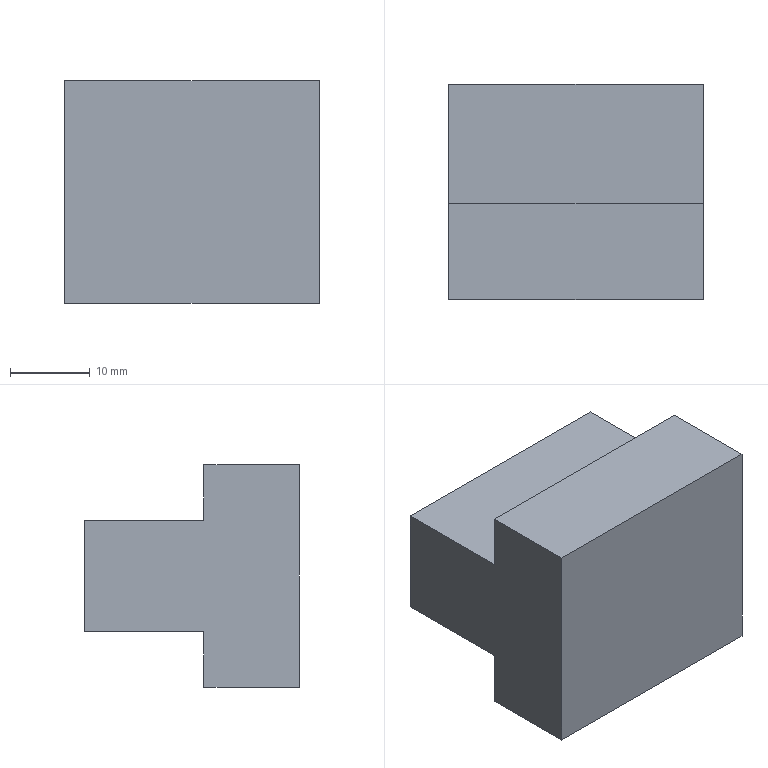Part | STEP file | PN_0009 gripper MHS3-80D | 1 solid | 18 faces | box 32 x 27 x 28 mm | volume 16863 mm3 | plane 10 | cylinder 4 | cone 4 | commonest cylinder face diameters 5 x4
STEP:
#1=CARTESIAN_POINT('',(0.,0.,0.));
#2=DIRECTION('',(0.,0.,1.));
#3=DIRECTION('',(1.,0.,0.));
#4=AXIS2_PLACEMENT_3D('',#1,#2,#3);
#5=CARTESIAN_POINT('',(-10.,12.,2.5));
#6=VERTEX_POINT('',#5);
#7=CARTESIAN_POINT('',(-10.,27.,2.5));
#8=VERTEX_POINT('',#7);
#9=CARTESIAN_POINT('',(-10.,27.,2.5));
#10=DIRECTION('',(0.,1.,0.));
#11=VECTOR('',#10,1.);
#12=LINE('',#9,#11);
#13=CARTESIAN_POINT('',(-10.,27.,0.));
#14=DIRECTION('',(0.,1.,0.));
#15=DIRECTION('',(0.,0.,1.));
#16=AXIS2_PLACEMENT_3D('',#13,#14,#15);
#17=CYLINDRICAL_SURFACE('',#16,2.5);
#18=CARTESIAN_POINT('',(6.283,0.));
#19=DIRECTION('',(0.,1.));
#20=VECTOR('',#19,1.);
#21=LINE('',#18,#20);
#22=(GEOMETRIC_REPRESENTATION_CONTEXT(2)PARAMETRIC_REPRESENTATION_CONTEXT()REPRESENTATION_CONTEXT('',''));
#23=DEFINITIONAL_REPRESENTATION('',(#21),#22);
#24=PCURVE('',#17,#23);
#25=CARTESIAN_POINT('',(-10.,27.,0.));
#26=DIRECTION('',(0.,1.,0.));
#27=DIRECTION('',(0.,0.,1.));
#28=AXIS2_PLACEMENT_3D('',#25,#26,#27);
#29=CYLINDRICAL_SURFACE('',#28,2.5);
#30=CARTESIAN_POINT('',(0.,0.));
#31=DIRECTION('',(0.,1.));
#32=VECTOR('',#31,1.);
#33=LINE('',#30,#32);
#34=(GEOMETRIC_REPRESENTATION_CONTEXT(2)PARAMETRIC_REPRESENTATION_CONTEXT()REPRESENTATION_CONTEXT('',''));
#35=DEFINITIONAL_REPRESENTATION('',(#33),#34);
#36=PCURVE('',#29,#35);
#37=SURFACE_CURVE('',#12,(#24,#36),.PCURVE_S1.);
#38=EDGE_CURVE('',#6,#8,#37,.T.);
#39=ORIENTED_EDGE('',*,*,#38,.T.);
#40=CARTESIAN_POINT('',(-10.,27.,-2.5));
#41=VERTEX_POINT('',#40);
#42=CARTESIAN_POINT('',(-10.,27.,0.));
#43=DIRECTION('',(0.,1.,0.));
#44=DIRECTION('',(0.,0.,1.));
#45=AXIS2_PLACEMENT_3D('',#42,#43,#44);
#46=CIRCLE('',#45,2.5);
#47=CARTESIAN_POINT('',(0.,0.));
#48=DIRECTION('',(1.,0.));
#49=VECTOR('',#48,1.);
#50=LINE('',#47,#49);
#51=(GEOMETRIC_REPRESENTATION_CONTEXT(2)PARAMETRIC_REPRESENTATION_CONTEXT()REPRESENTATION_CONTEXT('',''));
#52=DEFINITIONAL_REPRESENTATION('',(#50),#51);
#53=PCURVE('',#17,#52);
#54=CARTESIAN_POINT('',(16.,27.,7.));
#55=DIRECTION('',(0.,-1.,0.));
#56=DIRECTION('',(0.,0.,-1.));
#57=AXIS2_PLACEMENT_3D('',#54,#55,#56);
#58=PLANE('',#57);
#59=CARTESIAN_POINT('',(4.5,-26.));
#60=CARTESIAN_POINT('',(4.5,-21.67));
#61=CARTESIAN_POINT('',(8.25,-23.835));
#62=CARTESIAN_POINT('',(12.,-26.));
#63=CARTESIAN_POINT('',(8.25,-28.165));
#64=CARTESIAN_POINT('',(4.5,-30.33));
#65=CARTESIAN_POINT('',(4.5,-26.));
#66=(BOUNDED_CURVE()B_SPLINE_CURVE(2,(#59,#60,#61,#62,#63,#64,#65),.UNSPECIFIED.,.T.,.F.)B_SPLINE_CURVE_WITH_KNOTS((1,2,2,2,2,1),(-2.094,0.,2.094,4.189,6.283,8.378),.UNSPECIFIED.)CURVE()GEOMETRIC_REPRESENTATION_ITEM()RATIONAL_B_SPLINE_CURVE((1.,0.5,1.,0.5,1.,0.5,1.))REPRESENTATION_ITEM(''));
#67=(GEOMETRIC_REPRESENTATION_CONTEXT(2)PARAMETRIC_REPRESENTATION_CONTEXT()REPRESENTATION_CONTEXT('',''));
#68=DEFINITIONAL_REPRESENTATION('',(#66),#67);
#69=PCURVE('',#58,#68);
#70=SURFACE_CURVE('',#46,(#53,#69),.PCURVE_S1.);
#71=EDGE_CURVE('',#41,#8,#70,.T.);
#72=ORIENTED_EDGE('',*,*,#71,.F.);
#73=CARTESIAN_POINT('',(-10.,12.,-2.5));
#74=VERTEX_POINT('',#73);
#75=CARTESIAN_POINT('',(-10.,27.,-2.5));
#76=DIRECTION('',(0.,1.,0.));
#77=VECTOR('',#76,1.);
#78=LINE('',#75,#77);
#79=CARTESIAN_POINT('',(3.142,0.));
#80=DIRECTION('',(0.,1.));
#81=VECTOR('',#80,1.);
#82=LINE('',#79,#81);
#83=(GEOMETRIC_REPRESENTATION_CONTEXT(2)PARAMETRIC_REPRESENTATION_CONTEXT()REPRESENTATION_CONTEXT('',''));
#84=DEFINITIONAL_REPRESENTATION('',(#82),#83);
#85=PCURVE('',#17,#84);
#86=CARTESIAN_POINT('',(3.142,0.));
#87=DIRECTION('',(0.,1.));
#88=VECTOR('',#87,1.);
#89=LINE('',#86,#88);
#90=(GEOMETRIC_REPRESENTATION_CONTEXT(2)PARAMETRIC_REPRESENTATION_CONTEXT()REPRESENTATION_CONTEXT('',''));
#91=DEFINITIONAL_REPRESENTATION('',(#89),#90);
#92=PCURVE('',#29,#91);
#93=SURFACE_CURVE('',#78,(#85,#92),.PCURVE_S1.);
#94=EDGE_CURVE('',#74,#41,#93,.T.);
#95=ORIENTED_EDGE('',*,*,#94,.F.);
#96=CARTESIAN_POINT('',(-10.,12.,0.));
#97=DIRECTION('',(0.,1.,0.));
#98=DIRECTION('',(0.,0.,1.));
#99=AXIS2_PLACEMENT_3D('',#96,#97,#98);
#100=CIRCLE('',#99,2.5);
#101=CARTESIAN_POINT('',(0.,-15.));
#102=DIRECTION('',(1.,0.));
#103=VECTOR('',#102,1.);
#104=LINE('',#101,#103);
#105=(GEOMETRIC_REPRESENTATION_CONTEXT(2)PARAMETRIC_REPRESENTATION_CONTEXT()REPRESENTATION_CONTEXT('',''));
#106=DEFINITIONAL_REPRESENTATION('',(#104),#105);
#107=PCURVE('',#17,#106);
#108=CARTESIAN_POINT('',(-10.,12.,0.));
#109=DIRECTION('',(0.,1.,0.));
#110=DIRECTION('',(0.,0.,1.));
#111=AXIS2_PLACEMENT_3D('',#108,#109,#110);
#112=CONICAL_SURFACE('',#111,2.5,1.03);
#113=CARTESIAN_POINT('',(0.,0.));
#114=DIRECTION('',(1.,0.));
#115=VECTOR('',#114,1.);
#116=LINE('',#113,#115);
#117=(GEOMETRIC_REPRESENTATION_CONTEXT(2)PARAMETRIC_REPRESENTATION_CONTEXT()REPRESENTATION_CONTEXT('',''));
#118=DEFINITIONAL_REPRESENTATION('',(#116),#117);
#119=PCURVE('',#112,#118);
#120=SURFACE_CURVE('',#100,(#107,#119),.PCURVE_S1.);
#121=EDGE_CURVE('',#74,#6,#120,.T.);
#122=ORIENTED_EDGE('',*,*,#121,.T.);
#123=EDGE_LOOP('',(#39,#72,#95,#122));
#124=FACE_BOUND('',#123,.F.);
#125=ADVANCED_FACE('',(#124),#17,.F.);
#126=ORIENTED_EDGE('',*,*,#121,.F.);
#127=CARTESIAN_POINT('',(-10.,10.498,0.));
#128=VERTEX_POINT('',#127);
#129=CARTESIAN_POINT('',(-10.,12.,-2.5));
#130=DIRECTION('',(0.,0.515,-0.8572));
#131=VECTOR('',#130,1.);
#132=LINE('',#129,#131);
#133=CARTESIAN_POINT('',(3.142,0.));
#134=DIRECTION('',(0.,1.));
#135=VECTOR('',#134,1.);
#136=LINE('',#133,#135);
#137=(GEOMETRIC_REPRESENTATION_CONTEXT(2)PARAMETRIC_REPRESENTATION_CONTEXT()REPRESENTATION_CONTEXT('',''));
#138=DEFINITIONAL_REPRESENTATION('',(#136),#137);
#139=PCURVE('',#112,#138);
#140=CARTESIAN_POINT('',(-10.,12.,0.));
#141=DIRECTION('',(0.,1.,0.));
#142=DIRECTION('',(0.,0.,1.));
#143=AXIS2_PLACEMENT_3D('',#140,#141,#142);
#144=CONICAL_SURFACE('',#143,2.5,1.03);
#145=CARTESIAN_POINT('',(3.142,0.));
#146=DIRECTION('',(0.,1.));
#147=VECTOR('',#146,1.);
#148=LINE('',#145,#147);
#149=(GEOMETRIC_REPRESENTATION_CONTEXT(2)PARAMETRIC_REPRESENTATION_CONTEXT()REPRESENTATION_CONTEXT('',''));
#150=DEFINITIONAL_REPRESENTATION('',(#148),#149);
#151=PCURVE('',#144,#150);
#152=SURFACE_CURVE('',#132,(#139,#151),.PCURVE_S1.);
#153=EDGE_CURVE('',#128,#74,#152,.T.);
#154=ORIENTED_EDGE('',*,*,#153,.F.);
#155=CARTESIAN_POINT('',(-10.,12.,2.5));
#156=DIRECTION('',(0.,0.515,0.8572));
#157=VECTOR('',#156,1.);
#158=LINE('',#155,#157);
#159=CARTESIAN_POINT('',(6.283,0.));
#160=DIRECTION('',(0.,1.));
#161=VECTOR('',#160,1.);
#162=LINE('',#159,#161);
#163=(GEOMETRIC_REPRESENTATION_CONTEXT(2)PARAMETRIC_REPRESENTATION_CONTEXT()REPRESENTATION_CONTEXT('',''));
#164=DEFINITIONAL_REPRESENTATION('',(#162),#163);
#165=PCURVE('',#112,#164);
#166=CARTESIAN_POINT('',(0.,0.));
#167=DIRECTION('',(0.,1.));
#168=VECTOR('',#167,1.);
#169=LINE('',#166,#168);
#170=(GEOMETRIC_REPRESENTATION_CONTEXT(2)PARAMETRIC_REPRESENTATION_CONTEXT()REPRESENTATION_CONTEXT('',''));
#171=DEFINITIONAL_REPRESENTATION('',(#169),#170);
#172=PCURVE('',#144,#171);
#173=SURFACE_CURVE('',#158,(#165,#172),.PCURVE_S1.);
#174=EDGE_CURVE('',#128,#6,#173,.T.);
#175=ORIENTED_EDGE('',*,*,#174,.T.);
#176=EDGE_LOOP('',(#126,#154,#175));
#177=FACE_BOUND('',#176,.F.);
#178=ADVANCED_FACE('',(#177),#112,.F.);
#179=CARTESIAN_POINT('',(10.,12.,2.5));
#180=VERTEX_POINT('',#179);
#181=CARTESIAN_POINT('',(10.,27.,2.5));
#182=VERTEX_POINT('',#181);
#183=CARTESIAN_POINT('',(10.,27.,2.5));
#184=DIRECTION('',(0.,1.,0.));
#185=VECTOR('',#184,1.);
#186=LINE('',#183,#185);
#187=CARTESIAN_POINT('',(10.,27.,0.));
#188=DIRECTION('',(0.,1.,0.));
#189=DIRECTION('',(0.,0.,1.));
#190=AXIS2_PLACEMENT_3D('',#187,#188,#189);
#191=CYLINDRICAL_SURFACE('',#190,2.5);
#192=CARTESIAN_POINT('',(6.283,0.));
#193=DIRECTION('',(0.,1.));
#194=VECTOR('',#193,1.);
#195=LINE('',#192,#194);
#196=(GEOMETRIC_REPRESENTATION_CONTEXT(2)PARAMETRIC_REPRESENTATION_CONTEXT()REPRESENTATION_CONTEXT('',''));
#197=DEFINITIONAL_REPRESENTATION('',(#195),#196);
#198=PCURVE('',#191,#197);
#199=CARTESIAN_POINT('',(10.,27.,0.));
#200=DIRECTION('',(0.,1.,0.));
#201=DIRECTION('',(0.,0.,1.));
#202=AXIS2_PLACEMENT_3D('',#199,#200,#201);
#203=CYLINDRICAL_SURFACE('',#202,2.5);
#204=CARTESIAN_POINT('',(0.,0.));
#205=DIRECTION('',(0.,1.));
#206=VECTOR('',#205,1.);
#207=LINE('',#204,#206);
#208=(GEOMETRIC_REPRESENTATION_CONTEXT(2)PARAMETRIC_REPRESENTATION_CONTEXT()REPRESENTATION_CONTEXT('',''));
#209=DEFINITIONAL_REPRESENTATION('',(#207),#208);
#210=PCURVE('',#203,#209);
#211=SURFACE_CURVE('',#186,(#198,#210),.PCURVE_S1.);
#212=EDGE_CURVE('',#180,#182,#211,.T.);
#213=ORIENTED_EDGE('',*,*,#212,.T.);
#214=CARTESIAN_POINT('',(10.,27.,-2.5));
#215=VERTEX_POINT('',#214);
#216=CARTESIAN_POINT('',(10.,27.,0.));
#217=DIRECTION('',(0.,1.,0.));
#218=DIRECTION('',(0.,0.,1.));
#219=AXIS2_PLACEMENT_3D('',#216,#217,#218);
#220=CIRCLE('',#219,2.5);
#221=CARTESIAN_POINT('',(0.,0.));
#222=DIRECTION('',(1.,0.));
#223=VECTOR('',#222,1.);
#224=LINE('',#221,#223);
#225=(GEOMETRIC_REPRESENTATION_CONTEXT(2)PARAMETRIC_REPRESENTATION_CONTEXT()REPRESENTATION_CONTEXT('',''));
#226=DEFINITIONAL_REPRESENTATION('',(#224),#225);
#227=PCURVE('',#191,#226);
#228=CARTESIAN_POINT('',(4.5,-6.));
#229=CARTESIAN_POINT('',(4.5,-1.67));
#230=CARTESIAN_POINT('',(8.25,-3.835));
#231=CARTESIAN_POINT('',(12.,-6.));
#232=CARTESIAN_POINT('',(8.25,-8.165));
#233=CARTESIAN_POINT('',(4.5,-10.33));
#234=CARTESIAN_POINT('',(4.5,-6.));
#235=(BOUNDED_CURVE()B_SPLINE_CURVE(2,(#228,#229,#230,#231,#232,#233,#234),.UNSPECIFIED.,.T.,.F.)B_SPLINE_CURVE_WITH_KNOTS((1,2,2,2,2,1),(-2.094,0.,2.094,4.189,6.283,8.378),.UNSPECIFIED.)CURVE()GEOMETRIC_REPRESENTATION_ITEM()RATIONAL_B_SPLINE_CURVE((1.,0.5,1.,0.5,1.,0.5,1.))REPRESENTATION_ITEM(''));
#236=(GEOMETRIC_REPRESENTATION_CONTEXT(2)PARAMETRIC_REPRESENTATION_CONTEXT()REPRESENTATION_CONTEXT('',''));
#237=DEFINITIONAL_REPRESENTATION('',(#235),#236);
#238=PCURVE('',#58,#237);
#239=SURFACE_CURVE('',#220,(#227,#238),.PCURVE_S1.);
#240=EDGE_CURVE('',#215,#182,#239,.T.);
#241=ORIENTED_EDGE('',*,*,#240,.F.);
#242=CARTESIAN_POINT('',(10.,12.,-2.5));
#243=VERTEX_POINT('',#242);
#244=CARTESIAN_POINT('',(10.,27.,-2.5));
#245=DIRECTION('',(0.,1.,0.));
#246=VECTOR('',#245,1.);
#247=LINE('',#244,#246);
#248=CARTESIAN_POINT('',(3.142,0.));
#249=DIRECTION('',(0.,1.));
#250=VECTOR('',#249,1.);
#251=LINE('',#248,#250);
#252=(GEOMETRIC_REPRESENTATION_CONTEXT(2)PARAMETRIC_REPRESENTATION_CONTEXT()REPRESENTATION_CONTEXT('',''));
#253=DEFINITIONAL_REPRESENTATION('',(#251),#252);
#254=PCURVE('',#191,#253);
#255=CARTESIAN_POINT('',(3.142,0.));
#256=DIRECTION('',(0.,1.));
#257=VECTOR('',#256,1.);
#258=LINE('',#255,#257);
#259=(GEOMETRIC_REPRESENTATION_CONTEXT(2)PARAMETRIC_REPRESENTATION_CONTEXT()REPRESENTATION_CONTEXT('',''));
#260=DEFINITIONAL_REPRESENTATION('',(#258),#259);
#261=PCURVE('',#203,#260);
#262=SURFACE_CURVE('',#247,(#254,#261),.PCURVE_S1.);
#263=EDGE_CURVE('',#243,#215,#262,.T.);
#264=ORIENTED_EDGE('',*,*,#263,.F.);
#265=CARTESIAN_POINT('',(10.,12.,0.));
#266=DIRECTION('',(0.,1.,0.));
#267=DIRECTION('',(0.,0.,1.));
#268=AXIS2_PLACEMENT_3D('',#265,#266,#267);
#269=CIRCLE('',#268,2.5);
#270=CARTESIAN_POINT('',(0.,-15.));
#271=DIRECTION('',(1.,0.));
#272=VECTOR('',#271,1.);
#273=LINE('',#270,#272);
#274=(GEOMETRIC_REPRESENTATION_CONTEXT(2)PARAMETRIC_REPRESENTATION_CONTEXT()REPRESENTATION_CONTEXT('',''));
#275=DEFINITIONAL_REPRESENTATION('',(#273),#274);
#276=PCURVE('',#191,#275);
#277=CARTESIAN_POINT('',(10.,12.,0.));
#278=DIRECTION('',(0.,1.,0.));
#279=DIRECTION('',(0.,0.,1.));
#280=AXIS2_PLACEMENT_3D('',#277,#278,#279);
#281=CONICAL_SURFACE('',#280,2.5,1.03);
#282=CARTESIAN_POINT('',(0.,0.));
#283=DIRECTION('',(1.,0.));
#284=VECTOR('',#283,1.);
#285=LINE('',#282,#284);
#286=(GEOMETRIC_REPRESENTATION_CONTEXT(2)PARAMETRIC_REPRESENTATION_CONTEXT()REPRESENTATION_CONTEXT('',''));
#287=DEFINITIONAL_REPRESENTATION('',(#285),#286);
#288=PCURVE('',#281,#287);
#289=SURFACE_CURVE('',#269,(#276,#288),.PCURVE_S1.);
#290=EDGE_CURVE('',#243,#180,#289,.T.);
#291=ORIENTED_EDGE('',*,*,#290,.T.);
#292=EDGE_LOOP('',(#213,#241,#264,#291));
#293=FACE_BOUND('',#292,.F.);
#294=ADVANCED_FACE('',(#293),#191,.F.);
#295=ORIENTED_EDGE('',*,*,#290,.F.);
#296=CARTESIAN_POINT('',(10.,10.498,0.));
#297=VERTEX_POINT('',#296);
#298=CARTESIAN_POINT('',(10.,12.,-2.5));
#299=DIRECTION('',(0.,0.515,-0.8572));
#300=VECTOR('',#299,1.);
#301=LINE('',#298,#300);
#302=CARTESIAN_POINT('',(3.142,0.));
#303=DIRECTION('',(0.,1.));
#304=VECTOR('',#303,1.);
#305=LINE('',#302,#304);
#306=(GEOMETRIC_REPRESENTATION_CONTEXT(2)PARAMETRIC_REPRESENTATION_CONTEXT()REPRESENTATION_CONTEXT('',''));
#307=DEFINITIONAL_REPRESENTATION('',(#305),#306);
#308=PCURVE('',#281,#307);
#309=CARTESIAN_POINT('',(10.,12.,0.));
#310=DIRECTION('',(0.,1.,0.));
#311=DIRECTION('',(0.,0.,1.));
#312=AXIS2_PLACEMENT_3D('',#309,#310,#311);
#313=CONICAL_SURFACE('',#312,2.5,1.03);
#314=CARTESIAN_POINT('',(3.142,0.));
#315=DIRECTION('',(0.,1.));
#316=VECTOR('',#315,1.);
#317=LINE('',#314,#316);
#318=(GEOMETRIC_REPRESENTATION_CONTEXT(2)PARAMETRIC_REPRESENTATION_CONTEXT()REPRESENTATION_CONTEXT('',''));
#319=DEFINITIONAL_REPRESENTATION('',(#317),#318);
#320=PCURVE('',#313,#319);
#321=SURFACE_CURVE('',#301,(#308,#320),.PCURVE_S1.);
#322=EDGE_CURVE('',#297,#243,#321,.T.);
#323=ORIENTED_EDGE('',*,*,#322,.F.);
#324=CARTESIAN_POINT('',(10.,12.,2.5));
#325=DIRECTION('',(0.,0.515,0.8572));
#326=VECTOR('',#325,1.);
#327=LINE('',#324,#326);
#328=CARTESIAN_POINT('',(6.283,0.));
#329=DIRECTION('',(0.,1.));
#330=VECTOR('',#329,1.);
#331=LINE('',#328,#330);
#332=(GEOMETRIC_REPRESENTATION_CONTEXT(2)PARAMETRIC_REPRESENTATION_CONTEXT()REPRESENTATION_CONTEXT('',''));
#333=DEFINITIONAL_REPRESENTATION('',(#331),#332);
#334=PCURVE('',#281,#333);
#335=CARTESIAN_POINT('',(0.,0.));
#336=DIRECTION('',(0.,1.));
#337=VECTOR('',#336,1.);
#338=LINE('',#335,#337);
#339=(GEOMETRIC_REPRESENTATION_CONTEXT(2)PARAMETRIC_REPRESENTATION_CONTEXT()REPRESENTATION_CONTEXT('',''));
#340=DEFINITIONAL_REPRESENTATION('',(#338),#339);
#341=PCURVE('',#313,#340);
#342=SURFACE_CURVE('',#327,(#334,#341),.PCURVE_S1.);
#343=EDGE_CURVE('',#297,#180,#342,.T.);
#344=ORIENTED_EDGE('',*,*,#343,.T.);
#345=EDGE_LOOP('',(#295,#323,#344));
#346=FACE_BOUND('',#345,.F.);
#347=ADVANCED_FACE('',(#346),#281,.F.);
#348=CARTESIAN_POINT('',(-16.,12.,14.));
#349=VERTEX_POINT('',#348);
#350=CARTESIAN_POINT('',(-16.,0.,14.));
#351=VERTEX_POINT('',#350);
#352=CARTESIAN_POINT('',(-16.,0.,14.));
#353=DIRECTION('',(0.,-1.,0.));
#354=VECTOR('',#353,1.);
#355=LINE('',#352,#354);
#356=CARTESIAN_POINT('',(16.,0.,14.));
#357=DIRECTION('',(0.,0.,-1.));
#358=DIRECTION('',(-1.,0.,0.));
#359=AXIS2_PLACEMENT_3D('',#356,#357,#358);
#360=PLANE('',#359);
#361=CARTESIAN_POINT('',(32.,0.));
#362=DIRECTION('',(0.,-1.));
#363=VECTOR('',#362,1.);
#364=LINE('',#361,#363);
#365=(GEOMETRIC_REPRESENTATION_CONTEXT(2)PARAMETRIC_REPRESENTATION_CONTEXT()REPRESENTATION_CONTEXT('',''));
#366=DEFINITIONAL_REPRESENTATION('',(#364),#365);
#367=PCURVE('',#360,#366);
#368=CARTESIAN_POINT('',(-16.,0.,0.));
#369=DIRECTION('',(-1.,0.,0.));
#370=DIRECTION('',(0.,0.,1.));
#371=AXIS2_PLACEMENT_3D('',#368,#369,#370);
#372=PLANE('',#371);
#373=CARTESIAN_POINT('',(14.,0.));
#374=DIRECTION('',(0.,-1.));
#375=VECTOR('',#374,1.);
#376=LINE('',#373,#375);
#377=(GEOMETRIC_REPRESENTATION_CONTEXT(2)PARAMETRIC_REPRESENTATION_CONTEXT()REPRESENTATION_CONTEXT('',''));
#378=DEFINITIONAL_REPRESENTATION('',(#376),#377);
#379=PCURVE('',#372,#378);
#380=SURFACE_CURVE('',#355,(#367,#379),.PCURVE_S1.);
#381=EDGE_CURVE('',#349,#351,#380,.T.);
#382=ORIENTED_EDGE('',*,*,#381,.T.);
#383=CARTESIAN_POINT('',(16.,0.,14.));
#384=VERTEX_POINT('',#383);
#385=CARTESIAN_POINT('',(16.,0.,14.));
#386=DIRECTION('',(-1.,0.,0.));
#387=VECTOR('',#386,1.);
#388=LINE('',#385,#387);
#389=CARTESIAN_POINT('',(0.,0.));
#390=DIRECTION('',(1.,0.));
#391=VECTOR('',#390,1.);
#392=LINE('',#389,#391);
#393=(GEOMETRIC_REPRESENTATION_CONTEXT(2)PARAMETRIC_REPRESENTATION_CONTEXT()REPRESENTATION_CONTEXT('',''));
#394=DEFINITIONAL_REPRESENTATION('',(#392),#393);
#395=PCURVE('',#360,#394);
#396=CARTESIAN_POINT('',(16.,0.,14.));
#397=DIRECTION('',(0.,1.,0.));
#398=DIRECTION('',(0.,0.,1.));
#399=AXIS2_PLACEMENT_3D('',#396,#397,#398);
#400=PLANE('',#399);
#401=CARTESIAN_POINT('',(0.,0.));
#402=DIRECTION('',(0.,-1.));
#403=VECTOR('',#402,1.);
#404=LINE('',#401,#403);
#405=(GEOMETRIC_REPRESENTATION_CONTEXT(2)PARAMETRIC_REPRESENTATION_CONTEXT()REPRESENTATION_CONTEXT('',''));
#406=DEFINITIONAL_REPRESENTATION('',(#404),#405);
#407=PCURVE('',#400,#406);
#408=SURFACE_CURVE('',#388,(#395,#407),.PCURVE_S1.);
#409=EDGE_CURVE('',#384,#351,#408,.T.);
#410=ORIENTED_EDGE('',*,*,#409,.F.);
#411=CARTESIAN_POINT('',(16.,12.,14.));
#412=VERTEX_POINT('',#411);
#413=CARTESIAN_POINT('',(16.,0.,14.));
#414=DIRECTION('',(0.,-1.,0.));
#415=VECTOR('',#414,1.);
#416=LINE('',#413,#415);
#417=CARTESIAN_POINT('',(0.,0.));
#418=DIRECTION('',(0.,-1.));
#419=VECTOR('',#418,1.);
#420=LINE('',#417,#419);
#421=(GEOMETRIC_REPRESENTATION_CONTEXT(2)PARAMETRIC_REPRESENTATION_CONTEXT()REPRESENTATION_CONTEXT('',''));
#422=DEFINITIONAL_REPRESENTATION('',(#420),#421);
#423=PCURVE('',#360,#422);
#424=CARTESIAN_POINT('',(16.,0.,0.));
#425=DIRECTION('',(-1.,0.,0.));
#426=DIRECTION('',(0.,0.,1.));
#427=AXIS2_PLACEMENT_3D('',#424,#425,#426);
#428=PLANE('',#427);
#429=CARTESIAN_POINT('',(14.,0.));
#430=DIRECTION('',(0.,-1.));
#431=VECTOR('',#430,1.);
#432=LINE('',#429,#431);
#433=(GEOMETRIC_REPRESENTATION_CONTEXT(2)PARAMETRIC_REPRESENTATION_CONTEXT()REPRESENTATION_CONTEXT('',''));
#434=DEFINITIONAL_REPRESENTATION('',(#432),#433);
#435=PCURVE('',#428,#434);
#436=SURFACE_CURVE('',#416,(#423,#435),.PCURVE_S1.);
#437=EDGE_CURVE('',#412,#384,#436,.T.);
#438=ORIENTED_EDGE('',*,*,#437,.F.);
#439=CARTESIAN_POINT('',(16.,12.,14.));
#440=DIRECTION('',(-1.,0.,0.));
#441=VECTOR('',#440,1.);
#442=LINE('',#439,#441);
#443=CARTESIAN_POINT('',(0.,12.));
#444=DIRECTION('',(1.,0.));
#445=VECTOR('',#444,1.);
#446=LINE('',#443,#445);
#447=(GEOMETRIC_REPRESENTATION_CONTEXT(2)PARAMETRIC_REPRESENTATION_CONTEXT()REPRESENTATION_CONTEXT('',''));
#448=DEFINITIONAL_REPRESENTATION('',(#446),#447);
#449=PCURVE('',#360,#448);
#450=CARTESIAN_POINT('',(16.,12.,14.));
#451=DIRECTION('',(0.,-1.,0.));
#452=DIRECTION('',(0.,0.,-1.));
#453=AXIS2_PLACEMENT_3D('',#450,#451,#452);
#454=PLANE('',#453);
#455=CARTESIAN_POINT('',(0.,0.));
#456=DIRECTION('',(0.,-1.));
#457=VECTOR('',#456,1.);
#458=LINE('',#455,#457);
#459=(GEOMETRIC_REPRESENTATION_CONTEXT(2)PARAMETRIC_REPRESENTATION_CONTEXT()REPRESENTATION_CONTEXT('',''));
#460=DEFINITIONAL_REPRESENTATION('',(#458),#459);
#461=PCURVE('',#454,#460);
#462=SURFACE_CURVE('',#442,(#449,#461),.PCURVE_S1.);
#463=EDGE_CURVE('',#412,#349,#462,.T.);
#464=ORIENTED_EDGE('',*,*,#463,.T.);
#465=EDGE_LOOP('',(#382,#410,#438,#464));
#466=FACE_BOUND('',#465,.T.);
#467=ADVANCED_FACE('',(#466),#360,.F.);
#468=CARTESIAN_POINT('',(-16.,0.,-14.));
#469=VERTEX_POINT('',#468);
#470=CARTESIAN_POINT('',(-16.,0.,14.));
#471=DIRECTION('',(0.,0.,-1.));
#472=VECTOR('',#471,1.);
#473=LINE('',#470,#472);
#474=CARTESIAN_POINT('',(0.,-32.));
#475=DIRECTION('',(-1.,0.));
#476=VECTOR('',#475,1.);
#477=LINE('',#474,#476);
#478=(GEOMETRIC_REPRESENTATION_CONTEXT(2)PARAMETRIC_REPRESENTATION_CONTEXT()REPRESENTATION_CONTEXT('',''));
#479=DEFINITIONAL_REPRESENTATION('',(#477),#478);
#480=PCURVE('',#400,#479);
#481=CARTESIAN_POINT('',(14.,0.));
#482=DIRECTION('',(-1.,0.));
#483=VECTOR('',#482,1.);
#484=LINE('',#481,#483);
#485=(GEOMETRIC_REPRESENTATION_CONTEXT(2)PARAMETRIC_REPRESENTATION_CONTEXT()REPRESENTATION_CONTEXT('',''));
#486=DEFINITIONAL_REPRESENTATION('',(#484),#485);
#487=PCURVE('',#372,#486);
#488=SURFACE_CURVE('',#473,(#480,#487),.PCURVE_S1.);
#489=EDGE_CURVE('',#351,#469,#488,.T.);
#490=ORIENTED_EDGE('',*,*,#489,.T.);
#491=CARTESIAN_POINT('',(16.,0.,-14.));
#492=VERTEX_POINT('',#491);
#493=CARTESIAN_POINT('',(16.,0.,-14.));
#494=DIRECTION('',(-1.,0.,0.));
#495=VECTOR('',#494,1.);
#496=LINE('',#493,#495);
#497=CARTESIAN_POINT('',(-28.,0.));
#498=DIRECTION('',(0.,-1.));
#499=VECTOR('',#498,1.);
#500=LINE('',#497,#499);
#501=(GEOMETRIC_REPRESENTATION_CONTEXT(2)PARAMETRIC_REPRESENTATION_CONTEXT()REPRESENTATION_CONTEXT('',''));
#502=DEFINITIONAL_REPRESENTATION('',(#500),#501);
#503=PCURVE('',#400,#502);
#504=CARTESIAN_POINT('',(16.,0.,-14.));
#505=DIRECTION('',(0.,0.,1.));
#506=DIRECTION('',(1.,0.,0.));
#507=AXIS2_PLACEMENT_3D('',#504,#505,#506);
#508=PLANE('',#507);
#509=CARTESIAN_POINT('',(0.,0.));
#510=DIRECTION('',(-1.,0.));
#511=VECTOR('',#510,1.);
#512=LINE('',#509,#511);
#513=(GEOMETRIC_REPRESENTATION_CONTEXT(2)PARAMETRIC_REPRESENTATION_CONTEXT()REPRESENTATION_CONTEXT('',''));
#514=DEFINITIONAL_REPRESENTATION('',(#512),#513);
#515=PCURVE('',#508,#514);
#516=SURFACE_CURVE('',#496,(#503,#515),.PCURVE_S1.);
#517=EDGE_CURVE('',#492,#469,#516,.T.);
#518=ORIENTED_EDGE('',*,*,#517,.F.);
#519=CARTESIAN_POINT('',(16.,0.,14.));
#520=DIRECTION('',(0.,0.,-1.));
#521=VECTOR('',#520,1.);
#522=LINE('',#519,#521);
#523=CARTESIAN_POINT('',(0.,0.));
#524=DIRECTION('',(-1.,0.));
#525=VECTOR('',#524,1.);
#526=LINE('',#523,#525);
#527=(GEOMETRIC_REPRESENTATION_CONTEXT(2)PARAMETRIC_REPRESENTATION_CONTEXT()REPRESENTATION_CONTEXT('',''));
#528=DEFINITIONAL_REPRESENTATION('',(#526),#527);
#529=PCURVE('',#400,#528);
#530=CARTESIAN_POINT('',(14.,0.));
#531=DIRECTION('',(-1.,0.));
#532=VECTOR('',#531,1.);
#533=LINE('',#530,#532);
#534=(GEOMETRIC_REPRESENTATION_CONTEXT(2)PARAMETRIC_REPRESENTATION_CONTEXT()REPRESENTATION_CONTEXT('',''));
#535=DEFINITIONAL_REPRESENTATION('',(#533),#534);
#536=PCURVE('',#428,#535);
#537=SURFACE_CURVE('',#522,(#529,#536),.PCURVE_S1.);
#538=EDGE_CURVE('',#384,#492,#537,.T.);
#539=ORIENTED_EDGE('',*,*,#538,.F.);
#540=ORIENTED_EDGE('',*,*,#409,.T.);
#541=EDGE_LOOP('',(#490,#518,#539,#540));
#542=FACE_BOUND('',#541,.T.);
#543=ADVANCED_FACE('',(#542),#400,.F.);
#544=CARTESIAN_POINT('',(-16.,12.,-14.));
#545=VERTEX_POINT('',#544);
#546=CARTESIAN_POINT('',(-16.,0.,-14.));
#547=DIRECTION('',(0.,1.,0.));
#548=VECTOR('',#547,1.);
#549=LINE('',#546,#548);
#550=CARTESIAN_POINT('',(-32.,0.));
#551=DIRECTION('',(0.,1.));
#552=VECTOR('',#551,1.);
#553=LINE('',#550,#552);
#554=(GEOMETRIC_REPRESENTATION_CONTEXT(2)PARAMETRIC_REPRESENTATION_CONTEXT()REPRESENTATION_CONTEXT('',''));
#555=DEFINITIONAL_REPRESENTATION('',(#553),#554);
#556=PCURVE('',#508,#555);
#557=CARTESIAN_POINT('',(-14.,0.));
#558=DIRECTION('',(0.,1.));
#559=VECTOR('',#558,1.);
#560=LINE('',#557,#559);
#561=(GEOMETRIC_REPRESENTATION_CONTEXT(2)PARAMETRIC_REPRESENTATION_CONTEXT()REPRESENTATION_CONTEXT('',''));
#562=DEFINITIONAL_REPRESENTATION('',(#560),#561);
#563=PCURVE('',#372,#562);
#564=SURFACE_CURVE('',#549,(#556,#563),.PCURVE_S1.);
#565=EDGE_CURVE('',#469,#545,#564,.T.);
#566=ORIENTED_EDGE('',*,*,#565,.T.);
#567=CARTESIAN_POINT('',(16.,12.,-14.));
#568=VERTEX_POINT('',#567);
#569=CARTESIAN_POINT('',(16.,12.,-14.));
#570=DIRECTION('',(-1.,0.,0.));
#571=VECTOR('',#570,1.);
#572=LINE('',#569,#571);
#573=CARTESIAN_POINT('',(0.,12.));
#574=DIRECTION('',(-1.,0.));
#575=VECTOR('',#574,1.);
#576=LINE('',#573,#575);
#577=(GEOMETRIC_REPRESENTATION_CONTEXT(2)PARAMETRIC_REPRESENTATION_CONTEXT()REPRESENTATION_CONTEXT('',''));
#578=DEFINITIONAL_REPRESENTATION('',(#576),#577);
#579=PCURVE('',#508,#578);
#580=CARTESIAN_POINT('',(16.,12.,-7.));
#581=DIRECTION('',(0.,-1.,0.));
#582=DIRECTION('',(0.,0.,-1.));
#583=AXIS2_PLACEMENT_3D('',#580,#581,#582);
#584=PLANE('',#583);
#585=CARTESIAN_POINT('',(7.,0.));
#586=DIRECTION('',(0.,-1.));
#587=VECTOR('',#586,1.);
#588=LINE('',#585,#587);
#589=(GEOMETRIC_REPRESENTATION_CONTEXT(2)PARAMETRIC_REPRESENTATION_CONTEXT()REPRESENTATION_CONTEXT('',''));
#590=DEFINITIONAL_REPRESENTATION('',(#588),#589);
#591=PCURVE('',#584,#590);
#592=SURFACE_CURVE('',#572,(#579,#591),.PCURVE_S1.);
#593=EDGE_CURVE('',#568,#545,#592,.T.);
#594=ORIENTED_EDGE('',*,*,#593,.F.);
#595=CARTESIAN_POINT('',(16.,0.,-14.));
#596=DIRECTION('',(0.,1.,0.));
#597=VECTOR('',#596,1.);
#598=LINE('',#595,#597);
#599=CARTESIAN_POINT('',(0.,0.));
#600=DIRECTION('',(0.,1.));
#601=VECTOR('',#600,1.);
#602=LINE('',#599,#601);
#603=(GEOMETRIC_REPRESENTATION_CONTEXT(2)PARAMETRIC_REPRESENTATION_CONTEXT()REPRESENTATION_CONTEXT('',''));
#604=DEFINITIONAL_REPRESENTATION('',(#602),#603);
#605=PCURVE('',#508,#604);
#606=CARTESIAN_POINT('',(-14.,0.));
#607=DIRECTION('',(0.,1.));
#608=VECTOR('',#607,1.);
#609=LINE('',#606,#608);
#610=(GEOMETRIC_REPRESENTATION_CONTEXT(2)PARAMETRIC_REPRESENTATION_CONTEXT()REPRESENTATION_CONTEXT('',''));
#611=DEFINITIONAL_REPRESENTATION('',(#609),#610);
#612=PCURVE('',#428,#611);
#613=SURFACE_CURVE('',#598,(#605,#612),.PCURVE_S1.);
#614=EDGE_CURVE('',#492,#568,#613,.T.);
#615=ORIENTED_EDGE('',*,*,#614,.F.);
#616=ORIENTED_EDGE('',*,*,#517,.T.);
#617=EDGE_LOOP('',(#566,#594,#615,#616));
#618=FACE_BOUND('',#617,.T.);
#619=ADVANCED_FACE('',(#618),#508,.F.);
#620=CARTESIAN_POINT('',(-16.,12.,-7.));
#621=VERTEX_POINT('',#620);
#622=CARTESIAN_POINT('',(-16.,12.,-7.));
#623=DIRECTION('',(0.,0.,1.));
#624=VECTOR('',#623,1.);
#625=LINE('',#622,#624);
#626=CARTESIAN_POINT('',(0.,-32.));
#627=DIRECTION('',(-1.,0.));
#628=VECTOR('',#627,1.);
#629=LINE('',#626,#628);
#630=(GEOMETRIC_REPRESENTATION_CONTEXT(2)PARAMETRIC_REPRESENTATION_CONTEXT()REPRESENTATION_CONTEXT('',''));
#631=DEFINITIONAL_REPRESENTATION('',(#629),#630);
#632=PCURVE('',#584,#631);
#633=CARTESIAN_POINT('',(-7.,12.));
#634=DIRECTION('',(1.,0.));
#635=VECTOR('',#634,1.);
#636=LINE('',#633,#635);
#637=(GEOMETRIC_REPRESENTATION_CONTEXT(2)PARAMETRIC_REPRESENTATION_CONTEXT()REPRESENTATION_CONTEXT('',''));
#638=DEFINITIONAL_REPRESENTATION('',(#636),#637);
#639=PCURVE('',#372,#638);
#640=SURFACE_CURVE('',#625,(#632,#639),.PCURVE_S1.);
#641=EDGE_CURVE('',#545,#621,#640,.T.);
#642=ORIENTED_EDGE('',*,*,#641,.T.);
#643=CARTESIAN_POINT('',(16.,12.,-7.));
#644=VERTEX_POINT('',#643);
#645=CARTESIAN_POINT('',(16.,12.,-7.));
#646=DIRECTION('',(-1.,0.,0.));
#647=VECTOR('',#646,1.);
#648=LINE('',#645,#647);
#649=CARTESIAN_POINT('',(0.,0.));
#650=DIRECTION('',(0.,-1.));
#651=VECTOR('',#650,1.);
#652=LINE('',#649,#651);
#653=(GEOMETRIC_REPRESENTATION_CONTEXT(2)PARAMETRIC_REPRESENTATION_CONTEXT()REPRESENTATION_CONTEXT('',''));
#654=DEFINITIONAL_REPRESENTATION('',(#652),#653);
#655=PCURVE('',#584,#654);
#656=CARTESIAN_POINT('',(16.,27.,-7.));
#657=DIRECTION('',(0.,0.,1.));
#658=DIRECTION('',(0.,-1.,0.));
#659=AXIS2_PLACEMENT_3D('',#656,#657,#658);
#660=PLANE('',#659);
#661=CARTESIAN_POINT('',(15.,0.));
#662=DIRECTION('',(0.,-1.));
#663=VECTOR('',#662,1.);
#664=LINE('',#661,#663);
#665=(GEOMETRIC_REPRESENTATION_CONTEXT(2)PARAMETRIC_REPRESENTATION_CONTEXT()REPRESENTATION_CONTEXT('',''));
#666=DEFINITIONAL_REPRESENTATION('',(#664),#665);
#667=PCURVE('',#660,#666);
#668=SURFACE_CURVE('',#648,(#655,#667),.PCURVE_S1.);
#669=EDGE_CURVE('',#644,#621,#668,.T.);
#670=ORIENTED_EDGE('',*,*,#669,.F.);
#671=CARTESIAN_POINT('',(16.,12.,-7.));
#672=DIRECTION('',(0.,0.,1.));
#673=VECTOR('',#672,1.);
#674=LINE('',#671,#673);
#675=CARTESIAN_POINT('',(0.,0.));
#676=DIRECTION('',(-1.,0.));
#677=VECTOR('',#676,1.);
#678=LINE('',#675,#677);
#679=(GEOMETRIC_REPRESENTATION_CONTEXT(2)PARAMETRIC_REPRESENTATION_CONTEXT()REPRESENTATION_CONTEXT('',''));
#680=DEFINITIONAL_REPRESENTATION('',(#678),#679);
#681=PCURVE('',#584,#680);
#682=CARTESIAN_POINT('',(-7.,12.));
#683=DIRECTION('',(1.,0.));
#684=VECTOR('',#683,1.);
#685=LINE('',#682,#684);
#686=(GEOMETRIC_REPRESENTATION_CONTEXT(2)PARAMETRIC_REPRESENTATION_CONTEXT()REPRESENTATION_CONTEXT('',''));
#687=DEFINITIONAL_REPRESENTATION('',(#685),#686);
#688=PCURVE('',#428,#687);
#689=SURFACE_CURVE('',#674,(#681,#688),.PCURVE_S1.);
#690=EDGE_CURVE('',#568,#644,#689,.T.);
#691=ORIENTED_EDGE('',*,*,#690,.F.);
#692=ORIENTED_EDGE('',*,*,#593,.T.);
#693=EDGE_LOOP('',(#642,#670,#691,#692));
#694=FACE_BOUND('',#693,.T.);
#695=ADVANCED_FACE('',(#694),#584,.F.);
#696=CARTESIAN_POINT('',(-16.,27.,-7.));
#697=VERTEX_POINT('',#696);
#698=CARTESIAN_POINT('',(-16.,27.,-7.));
#699=DIRECTION('',(0.,1.,0.));
#700=VECTOR('',#699,1.);
#701=LINE('',#698,#700);
#702=CARTESIAN_POINT('',(0.,-32.));
#703=DIRECTION('',(-1.,0.));
#704=VECTOR('',#703,1.);
#705=LINE('',#702,#704);
#706=(GEOMETRIC_REPRESENTATION_CONTEXT(2)PARAMETRIC_REPRESENTATION_CONTEXT()REPRESENTATION_CONTEXT('',''));
#707=DEFINITIONAL_REPRESENTATION('',(#705),#706);
#708=PCURVE('',#660,#707);
#709=CARTESIAN_POINT('',(-7.,27.));
#710=DIRECTION('',(0.,1.));
#711=VECTOR('',#710,1.);
#712=LINE('',#709,#711);
#713=(GEOMETRIC_REPRESENTATION_CONTEXT(2)PARAMETRIC_REPRESENTATION_CONTEXT()REPRESENTATION_CONTEXT('',''));
#714=DEFINITIONAL_REPRESENTATION('',(#712),#713);
#715=PCURVE('',#372,#714);
#716=SURFACE_CURVE('',#701,(#708,#715),.PCURVE_S1.);
#717=EDGE_CURVE('',#621,#697,#716,.T.);
#718=ORIENTED_EDGE('',*,*,#717,.T.);
#719=CARTESIAN_POINT('',(16.,27.,-7.));
#720=VERTEX_POINT('',#719);
#721=CARTESIAN_POINT('',(16.,27.,-7.));
#722=DIRECTION('',(-1.,0.,0.));
#723=VECTOR('',#722,1.);
#724=LINE('',#721,#723);
#725=CARTESIAN_POINT('',(0.,0.));
#726=DIRECTION('',(0.,-1.));
#727=VECTOR('',#726,1.);
#728=LINE('',#725,#727);
#729=(GEOMETRIC_REPRESENTATION_CONTEXT(2)PARAMETRIC_REPRESENTATION_CONTEXT()REPRESENTATION_CONTEXT('',''));
#730=DEFINITIONAL_REPRESENTATION('',(#728),#729);
#731=PCURVE('',#660,#730);
#732=CARTESIAN_POINT('',(14.,0.));
#733=DIRECTION('',(0.,-1.));
#734=VECTOR('',#733,1.);
#735=LINE('',#732,#734);
#736=(GEOMETRIC_REPRESENTATION_CONTEXT(2)PARAMETRIC_REPRESENTATION_CONTEXT()REPRESENTATION_CONTEXT('',''));
#737=DEFINITIONAL_REPRESENTATION('',(#735),#736);
#738=PCURVE('',#58,#737);
#739=SURFACE_CURVE('',#724,(#731,#738),.PCURVE_S1.);
#740=EDGE_CURVE('',#720,#697,#739,.T.);
#741=ORIENTED_EDGE('',*,*,#740,.F.);
#742=CARTESIAN_POINT('',(16.,27.,-7.));
#743=DIRECTION('',(0.,1.,0.));
#744=VECTOR('',#743,1.);
#745=LINE('',#742,#744);
#746=CARTESIAN_POINT('',(0.,0.));
#747=DIRECTION('',(-1.,0.));
#748=VECTOR('',#747,1.);
#749=LINE('',#746,#748);
#750=(GEOMETRIC_REPRESENTATION_CONTEXT(2)PARAMETRIC_REPRESENTATION_CONTEXT()REPRESENTATION_CONTEXT('',''));
#751=DEFINITIONAL_REPRESENTATION('',(#749),#750);
#752=PCURVE('',#660,#751);
#753=CARTESIAN_POINT('',(-7.,27.));
#754=DIRECTION('',(0.,1.));
#755=VECTOR('',#754,1.);
#756=LINE('',#753,#755);
#757=(GEOMETRIC_REPRESENTATION_CONTEXT(2)PARAMETRIC_REPRESENTATION_CONTEXT()REPRESENTATION_CONTEXT('',''));
#758=DEFINITIONAL_REPRESENTATION('',(#756),#757);
#759=PCURVE('',#428,#758);
#760=SURFACE_CURVE('',#745,(#752,#759),.PCURVE_S1.);
#761=EDGE_CURVE('',#644,#720,#760,.T.);
#762=ORIENTED_EDGE('',*,*,#761,.F.);
#763=ORIENTED_EDGE('',*,*,#669,.T.);
#764=EDGE_LOOP('',(#718,#741,#762,#763));
#765=FACE_BOUND('',#764,.T.);
#766=ADVANCED_FACE('',(#765),#660,.F.);
#767=CARTESIAN_POINT('',(-10.,27.,0.));
#768=DIRECTION('',(0.,1.,0.));
#769=DIRECTION('',(0.,0.,1.));
#770=AXIS2_PLACEMENT_3D('',#767,#768,#769);
#771=CIRCLE('',#770,2.5);
#772=CARTESIAN_POINT('',(4.5,-26.));
#773=CARTESIAN_POINT('',(4.5,-21.67));
#774=CARTESIAN_POINT('',(8.25,-23.835));
#775=CARTESIAN_POINT('',(12.,-26.));
#776=CARTESIAN_POINT('',(8.25,-28.165));
#777=CARTESIAN_POINT('',(4.5,-30.33));
#778=CARTESIAN_POINT('',(4.5,-26.));
#779=(BOUNDED_CURVE()B_SPLINE_CURVE(2,(#772,#773,#774,#775,#776,#777,#778),.UNSPECIFIED.,.T.,.F.)B_SPLINE_CURVE_WITH_KNOTS((1,2,2,2,2,1),(-2.094,0.,2.094,4.189,6.283,8.378),.UNSPECIFIED.)CURVE()GEOMETRIC_REPRESENTATION_ITEM()RATIONAL_B_SPLINE_CURVE((1.,0.5,1.,0.5,1.,0.5,1.))REPRESENTATION_ITEM(''));
#780=(GEOMETRIC_REPRESENTATION_CONTEXT(2)PARAMETRIC_REPRESENTATION_CONTEXT()REPRESENTATION_CONTEXT('',''));
#781=DEFINITIONAL_REPRESENTATION('',(#779),#780);
#782=PCURVE('',#58,#781);
#783=CARTESIAN_POINT('',(0.,0.));
#784=DIRECTION('',(1.,0.));
#785=VECTOR('',#784,1.);
#786=LINE('',#783,#785);
#787=(GEOMETRIC_REPRESENTATION_CONTEXT(2)PARAMETRIC_REPRESENTATION_CONTEXT()REPRESENTATION_CONTEXT('',''));
#788=DEFINITIONAL_REPRESENTATION('',(#786),#787);
#789=PCURVE('',#29,#788);
#790=SURFACE_CURVE('',#771,(#782,#789),.PCURVE_S1.);
#791=EDGE_CURVE('',#8,#41,#790,.T.);
#792=ORIENTED_EDGE('',*,*,#791,.F.);
#793=ORIENTED_EDGE('',*,*,#71,.F.);
#794=EDGE_LOOP('',(#792,#793));
#795=FACE_BOUND('',#794,.T.);
#796=CARTESIAN_POINT('',(10.,27.,0.));
#797=DIRECTION('',(0.,1.,0.));
#798=DIRECTION('',(0.,0.,1.));
#799=AXIS2_PLACEMENT_3D('',#796,#797,#798);
#800=CIRCLE('',#799,2.5);
#801=CARTESIAN_POINT('',(4.5,-6.));
#802=CARTESIAN_POINT('',(4.5,-1.67));
#803=CARTESIAN_POINT('',(8.25,-3.835));
#804=CARTESIAN_POINT('',(12.,-6.));
#805=CARTESIAN_POINT('',(8.25,-8.165));
#806=CARTESIAN_POINT('',(4.5,-10.33));
#807=CARTESIAN_POINT('',(4.5,-6.));
#808=(BOUNDED_CURVE()B_SPLINE_CURVE(2,(#801,#802,#803,#804,#805,#806,#807),.UNSPECIFIED.,.T.,.F.)B_SPLINE_CURVE_WITH_KNOTS((1,2,2,2,2,1),(-2.094,0.,2.094,4.189,6.283,8.378),.UNSPECIFIED.)CURVE()GEOMETRIC_REPRESENTATION_ITEM()RATIONAL_B_SPLINE_CURVE((1.,0.5,1.,0.5,1.,0.5,1.))REPRESENTATION_ITEM(''));
#809=(GEOMETRIC_REPRESENTATION_CONTEXT(2)PARAMETRIC_REPRESENTATION_CONTEXT()REPRESENTATION_CONTEXT('',''));
#810=DEFINITIONAL_REPRESENTATION('',(#808),#809);
#811=PCURVE('',#58,#810);
#812=CARTESIAN_POINT('',(0.,0.));
#813=DIRECTION('',(1.,0.));
#814=VECTOR('',#813,1.);
#815=LINE('',#812,#814);
#816=(GEOMETRIC_REPRESENTATION_CONTEXT(2)PARAMETRIC_REPRESENTATION_CONTEXT()REPRESENTATION_CONTEXT('',''));
#817=DEFINITIONAL_REPRESENTATION('',(#815),#816);
#818=PCURVE('',#203,#817);
#819=SURFACE_CURVE('',#800,(#811,#818),.PCURVE_S1.);
#820=EDGE_CURVE('',#182,#215,#819,.T.);
#821=ORIENTED_EDGE('',*,*,#820,.F.);
#822=ORIENTED_EDGE('',*,*,#240,.F.);
#823=EDGE_LOOP('',(#821,#822));
#824=FACE_BOUND('',#823,.T.);
#825=CARTESIAN_POINT('',(-16.,27.,7.));
#826=VERTEX_POINT('',#825);
#827=CARTESIAN_POINT('',(-16.,27.,7.));
#828=DIRECTION('',(0.,0.,1.));
#829=VECTOR('',#828,1.);
#830=LINE('',#827,#829);
#831=CARTESIAN_POINT('',(0.,-32.));
#832=DIRECTION('',(-1.,0.));
#833=VECTOR('',#832,1.);
#834=LINE('',#831,#833);
#835=(GEOMETRIC_REPRESENTATION_CONTEXT(2)PARAMETRIC_REPRESENTATION_CONTEXT()REPRESENTATION_CONTEXT('',''));
#836=DEFINITIONAL_REPRESENTATION('',(#834),#835);
#837=PCURVE('',#58,#836);
#838=CARTESIAN_POINT('',(7.,27.));
#839=DIRECTION('',(1.,0.));
#840=VECTOR('',#839,1.);
#841=LINE('',#838,#840);
#842=(GEOMETRIC_REPRESENTATION_CONTEXT(2)PARAMETRIC_REPRESENTATION_CONTEXT()REPRESENTATION_CONTEXT('',''));
#843=DEFINITIONAL_REPRESENTATION('',(#841),#842);
#844=PCURVE('',#372,#843);
#845=SURFACE_CURVE('',#830,(#837,#844),.PCURVE_S1.);
#846=EDGE_CURVE('',#697,#826,#845,.T.);
#847=ORIENTED_EDGE('',*,*,#846,.T.);
#848=CARTESIAN_POINT('',(16.,27.,7.));
#849=VERTEX_POINT('',#848);
#850=CARTESIAN_POINT('',(16.,27.,7.));
#851=DIRECTION('',(-1.,0.,0.));
#852=VECTOR('',#851,1.);
#853=LINE('',#850,#852);
#854=CARTESIAN_POINT('',(0.,0.));
#855=DIRECTION('',(0.,-1.));
#856=VECTOR('',#855,1.);
#857=LINE('',#854,#856);
#858=(GEOMETRIC_REPRESENTATION_CONTEXT(2)PARAMETRIC_REPRESENTATION_CONTEXT()REPRESENTATION_CONTEXT('',''));
#859=DEFINITIONAL_REPRESENTATION('',(#857),#858);
#860=PCURVE('',#58,#859);
#861=CARTESIAN_POINT('',(16.,12.,7.));
#862=DIRECTION('',(0.,0.,-1.));
#863=DIRECTION('',(0.,1.,0.));
#864=AXIS2_PLACEMENT_3D('',#861,#862,#863);
#865=PLANE('',#864);
#866=CARTESIAN_POINT('',(15.,0.));
#867=DIRECTION('',(0.,-1.));
#868=VECTOR('',#867,1.);
#869=LINE('',#866,#868);
#870=(GEOMETRIC_REPRESENTATION_CONTEXT(2)PARAMETRIC_REPRESENTATION_CONTEXT()REPRESENTATION_CONTEXT('',''));
#871=DEFINITIONAL_REPRESENTATION('',(#869),#870);
#872=PCURVE('',#865,#871);
#873=SURFACE_CURVE('',#853,(#860,#872),.PCURVE_S1.);
#874=EDGE_CURVE('',#849,#826,#873,.T.);
#875=ORIENTED_EDGE('',*,*,#874,.F.);
#876=CARTESIAN_POINT('',(16.,27.,7.));
#877=DIRECTION('',(0.,0.,1.));
#878=VECTOR('',#877,1.);
#879=LINE('',#876,#878);
#880=CARTESIAN_POINT('',(0.,0.));
#881=DIRECTION('',(-1.,0.));
#882=VECTOR('',#881,1.);
#883=LINE('',#880,#882);
#884=(GEOMETRIC_REPRESENTATION_CONTEXT(2)PARAMETRIC_REPRESENTATION_CONTEXT()REPRESENTATION_CONTEXT('',''));
#885=DEFINITIONAL_REPRESENTATION('',(#883),#884);
#886=PCURVE('',#58,#885);
#887=CARTESIAN_POINT('',(7.,27.));
#888=DIRECTION('',(1.,0.));
#889=VECTOR('',#888,1.);
#890=LINE('',#887,#889);
#891=(GEOMETRIC_REPRESENTATION_CONTEXT(2)PARAMETRIC_REPRESENTATION_CONTEXT()REPRESENTATION_CONTEXT('',''));
#892=DEFINITIONAL_REPRESENTATION('',(#890),#891);
#893=PCURVE('',#428,#892);
#894=SURFACE_CURVE('',#879,(#886,#893),.PCURVE_S1.);
#895=EDGE_CURVE('',#720,#849,#894,.T.);
#896=ORIENTED_EDGE('',*,*,#895,.F.);
#897=ORIENTED_EDGE('',*,*,#740,.T.);
#898=EDGE_LOOP('',(#847,#875,#896,#897));
#899=FACE_BOUND('',#898,.T.);
#900=ADVANCED_FACE('',(#795,#824,#899),#58,.F.);
#901=CARTESIAN_POINT('',(-16.,12.,7.));
#902=VERTEX_POINT('',#901);
#903=CARTESIAN_POINT('',(-16.,12.,7.));
#904=DIRECTION('',(0.,-1.,0.));
#905=VECTOR('',#904,1.);
#906=LINE('',#903,#905);
#907=CARTESIAN_POINT('',(0.,-32.));
#908=DIRECTION('',(-1.,0.));
#909=VECTOR('',#908,1.);
#910=LINE('',#907,#909);
#911=(GEOMETRIC_REPRESENTATION_CONTEXT(2)PARAMETRIC_REPRESENTATION_CONTEXT()REPRESENTATION_CONTEXT('',''));
#912=DEFINITIONAL_REPRESENTATION('',(#910),#911);
#913=PCURVE('',#865,#912);
#914=CARTESIAN_POINT('',(7.,12.));
#915=DIRECTION('',(0.,-1.));
#916=VECTOR('',#915,1.);
#917=LINE('',#914,#916);
#918=(GEOMETRIC_REPRESENTATION_CONTEXT(2)PARAMETRIC_REPRESENTATION_CONTEXT()REPRESENTATION_CONTEXT('',''));
#919=DEFINITIONAL_REPRESENTATION('',(#917),#918);
#920=PCURVE('',#372,#919);
#921=SURFACE_CURVE('',#906,(#913,#920),.PCURVE_S1.);
#922=EDGE_CURVE('',#826,#902,#921,.T.);
#923=ORIENTED_EDGE('',*,*,#922,.T.);
#924=CARTESIAN_POINT('',(16.,12.,7.));
#925=VERTEX_POINT('',#924);
#926=CARTESIAN_POINT('',(16.,12.,7.));
#927=DIRECTION('',(-1.,0.,0.));
#928=VECTOR('',#927,1.);
#929=LINE('',#926,#928);
#930=CARTESIAN_POINT('',(0.,0.));
#931=DIRECTION('',(0.,-1.));
#932=VECTOR('',#931,1.);
#933=LINE('',#930,#932);
#934=(GEOMETRIC_REPRESENTATION_CONTEXT(2)PARAMETRIC_REPRESENTATION_CONTEXT()REPRESENTATION_CONTEXT('',''));
#935=DEFINITIONAL_REPRESENTATION('',(#933),#934);
#936=PCURVE('',#865,#935);
#937=CARTESIAN_POINT('',(7.,0.));
#938=DIRECTION('',(0.,-1.));
#939=VECTOR('',#938,1.);
#940=LINE('',#937,#939);
#941=(GEOMETRIC_REPRESENTATION_CONTEXT(2)PARAMETRIC_REPRESENTATION_CONTEXT()REPRESENTATION_CONTEXT('',''));
#942=DEFINITIONAL_REPRESENTATION('',(#940),#941);
#943=PCURVE('',#454,#942);
#944=SURFACE_CURVE('',#929,(#936,#943),.PCURVE_S1.);
#945=EDGE_CURVE('',#925,#902,#944,.T.);
#946=ORIENTED_EDGE('',*,*,#945,.F.);
#947=CARTESIAN_POINT('',(16.,12.,7.));
#948=DIRECTION('',(0.,-1.,0.));
#949=VECTOR('',#948,1.);
#950=LINE('',#947,#949);
#951=CARTESIAN_POINT('',(0.,0.));
#952=DIRECTION('',(-1.,0.));
#953=VECTOR('',#952,1.);
#954=LINE('',#951,#953);
#955=(GEOMETRIC_REPRESENTATION_CONTEXT(2)PARAMETRIC_REPRESENTATION_CONTEXT()REPRESENTATION_CONTEXT('',''));
#956=DEFINITIONAL_REPRESENTATION('',(#954),#955);
#957=PCURVE('',#865,#956);
#958=CARTESIAN_POINT('',(7.,12.));
#959=DIRECTION('',(0.,-1.));
#960=VECTOR('',#959,1.);
#961=LINE('',#958,#960);
#962=(GEOMETRIC_REPRESENTATION_CONTEXT(2)PARAMETRIC_REPRESENTATION_CONTEXT()REPRESENTATION_CONTEXT('',''));
#963=DEFINITIONAL_REPRESENTATION('',(#961),#962);
#964=PCURVE('',#428,#963);
#965=SURFACE_CURVE('',#950,(#957,#964),.PCURVE_S1.);
#966=EDGE_CURVE('',#849,#925,#965,.T.);
#967=ORIENTED_EDGE('',*,*,#966,.F.);
#968=ORIENTED_EDGE('',*,*,#874,.T.);
#969=EDGE_LOOP('',(#923,#946,#967,#968));
#970=FACE_BOUND('',#969,.T.);
#971=ADVANCED_FACE('',(#970),#865,.F.);
#972=CARTESIAN_POINT('',(-16.,12.,14.));
#973=DIRECTION('',(0.,0.,1.));
#974=VECTOR('',#973,1.);
#975=LINE('',#972,#974);
#976=CARTESIAN_POINT('',(0.,-32.));
#977=DIRECTION('',(-1.,0.));
#978=VECTOR('',#977,1.);
#979=LINE('',#976,#978);
#980=(GEOMETRIC_REPRESENTATION_CONTEXT(2)PARAMETRIC_REPRESENTATION_CONTEXT()REPRESENTATION_CONTEXT('',''));
#981=DEFINITIONAL_REPRESENTATION('',(#979),#980);
#982=PCURVE('',#454,#981);
#983=CARTESIAN_POINT('',(14.,12.));
#984=DIRECTION('',(1.,0.));
#985=VECTOR('',#984,1.);
#986=LINE('',#983,#985);
#987=(GEOMETRIC_REPRESENTATION_CONTEXT(2)PARAMETRIC_REPRESENTATION_CONTEXT()REPRESENTATION_CONTEXT('',''));
#988=DEFINITIONAL_REPRESENTATION('',(#986),#987);
#989=PCURVE('',#372,#988);
#990=SURFACE_CURVE('',#975,(#982,#989),.PCURVE_S1.);
#991=EDGE_CURVE('',#902,#349,#990,.T.);
#992=ORIENTED_EDGE('',*,*,#991,.T.);
#993=ORIENTED_EDGE('',*,*,#463,.F.);
#994=CARTESIAN_POINT('',(16.,12.,14.));
#995=DIRECTION('',(0.,0.,1.));
#996=VECTOR('',#995,1.);
#997=LINE('',#994,#996);
#998=CARTESIAN_POINT('',(0.,0.));
#999=DIRECTION('',(-1.,0.));
#1000=VECTOR('',#999,1.);
#1001=LINE('',#998,#1000);
#1002=(GEOMETRIC_REPRESENTATION_CONTEXT(2)PARAMETRIC_REPRESENTATION_CONTEXT()REPRESENTATION_CONTEXT('',''));
#1003=DEFINITIONAL_REPRESENTATION('',(#1001),#1002);
#1004=PCURVE('',#454,#1003);
#1005=CARTESIAN_POINT('',(14.,12.));
#1006=DIRECTION('',(1.,0.));
#1007=VECTOR('',#1006,1.);
#1008=LINE('',#1005,#1007);
#1009=(GEOMETRIC_REPRESENTATION_CONTEXT(2)PARAMETRIC_REPRESENTATION_CONTEXT()REPRESENTATION_CONTEXT('',''));
#1010=DEFINITIONAL_REPRESENTATION('',(#1008),#1009);
#1011=PCURVE('',#428,#1010);
#1012=SURFACE_CURVE('',#997,(#1004,#1011),.PCURVE_S1.);
#1013=EDGE_CURVE('',#925,#412,#1012,.T.);
#1014=ORIENTED_EDGE('',*,*,#1013,.F.);
#1015=ORIENTED_EDGE('',*,*,#945,.T.);
#1016=EDGE_LOOP('',(#992,#993,#1014,#1015));
#1017=FACE_BOUND('',#1016,.T.);
#1018=ADVANCED_FACE('',(#1017),#454,.F.);
#1019=ORIENTED_EDGE('',*,*,#437,.T.);
#1020=ORIENTED_EDGE('',*,*,#538,.T.);
#1021=ORIENTED_EDGE('',*,*,#614,.T.);
#1022=ORIENTED_EDGE('',*,*,#690,.T.);
#1023=ORIENTED_EDGE('',*,*,#761,.T.);
#1024=ORIENTED_EDGE('',*,*,#895,.T.);
#1025=ORIENTED_EDGE('',*,*,#966,.T.);
#1026=ORIENTED_EDGE('',*,*,#1013,.T.);
#1027=EDGE_LOOP('',(#1019,#1020,#1021,#1022,#1023,#1024,#1025,#1026));
#1028=FACE_BOUND('',#1027,.T.);
#1029=ADVANCED_FACE('',(#1028),#428,.F.);
#1030=ORIENTED_EDGE('',*,*,#381,.F.);
#1031=ORIENTED_EDGE('',*,*,#991,.F.);
#1032=ORIENTED_EDGE('',*,*,#922,.F.);
#1033=ORIENTED_EDGE('',*,*,#846,.F.);
#1034=ORIENTED_EDGE('',*,*,#717,.F.);
#1035=ORIENTED_EDGE('',*,*,#641,.F.);
#1036=ORIENTED_EDGE('',*,*,#565,.F.);
#1037=ORIENTED_EDGE('',*,*,#489,.F.);
#1038=EDGE_LOOP('',(#1030,#1031,#1032,#1033,#1034,#1035,#1036,#1037));
#1039=FACE_BOUND('',#1038,.T.);
#1040=ADVANCED_FACE('',(#1039),#372,.T.);
#1041=CARTESIAN_POINT('',(10.,12.,0.));
#1042=DIRECTION('',(0.,1.,0.));
#1043=DIRECTION('',(0.,0.,1.));
#1044=AXIS2_PLACEMENT_3D('',#1041,#1042,#1043);
#1045=CIRCLE('',#1044,2.5);
#1046=CARTESIAN_POINT('',(0.,0.));
#1047=DIRECTION('',(1.,0.));
#1048=VECTOR('',#1047,1.);
#1049=LINE('',#1046,#1048);
#1050=(GEOMETRIC_REPRESENTATION_CONTEXT(2)PARAMETRIC_REPRESENTATION_CONTEXT()REPRESENTATION_CONTEXT('',''));
#1051=DEFINITIONAL_REPRESENTATION('',(#1049),#1050);
#1052=PCURVE('',#313,#1051);
#1053=CARTESIAN_POINT('',(0.,-15.));
#1054=DIRECTION('',(1.,0.));
#1055=VECTOR('',#1054,1.);
#1056=LINE('',#1053,#1055);
#1057=(GEOMETRIC_REPRESENTATION_CONTEXT(2)PARAMETRIC_REPRESENTATION_CONTEXT()REPRESENTATION_CONTEXT('',''));
#1058=DEFINITIONAL_REPRESENTATION('',(#1056),#1057);
#1059=PCURVE('',#203,#1058);
#1060=SURFACE_CURVE('',#1045,(#1052,#1059),.PCURVE_S1.);
#1061=EDGE_CURVE('',#180,#243,#1060,.T.);
#1062=ORIENTED_EDGE('',*,*,#1061,.F.);
#1063=ORIENTED_EDGE('',*,*,#343,.F.);
#1064=ORIENTED_EDGE('',*,*,#322,.T.);
#1065=EDGE_LOOP('',(#1062,#1063,#1064));
#1066=FACE_BOUND('',#1065,.F.);
#1067=ADVANCED_FACE('',(#1066),#313,.F.);
#1068=ORIENTED_EDGE('',*,*,#820,.F.);
#1069=ORIENTED_EDGE('',*,*,#212,.F.);
#1070=ORIENTED_EDGE('',*,*,#1061,.T.);
#1071=ORIENTED_EDGE('',*,*,#263,.T.);
#1072=EDGE_LOOP('',(#1068,#1069,#1070,#1071));
#1073=FACE_BOUND('',#1072,.F.);
#1074=ADVANCED_FACE('',(#1073),#203,.F.);
#1075=CARTESIAN_POINT('',(-10.,12.,0.));
#1076=DIRECTION('',(0.,1.,0.));
#1077=DIRECTION('',(0.,0.,1.));
#1078=AXIS2_PLACEMENT_3D('',#1075,#1076,#1077);
#1079=CIRCLE('',#1078,2.5);
#1080=CARTESIAN_POINT('',(0.,0.));
#1081=DIRECTION('',(1.,0.));
#1082=VECTOR('',#1081,1.);
#1083=LINE('',#1080,#1082);
#1084=(GEOMETRIC_REPRESENTATION_CONTEXT(2)PARAMETRIC_REPRESENTATION_CONTEXT()REPRESENTATION_CONTEXT('',''));
#1085=DEFINITIONAL_REPRESENTATION('',(#1083),#1084);
#1086=PCURVE('',#144,#1085);
#1087=CARTESIAN_POINT('',(0.,-15.));
#1088=DIRECTION('',(1.,0.));
#1089=VECTOR('',#1088,1.);
#1090=LINE('',#1087,#1089);
#1091=(GEOMETRIC_REPRESENTATION_CONTEXT(2)PARAMETRIC_REPRESENTATION_CONTEXT()REPRESENTATION_CONTEXT('',''));
#1092=DEFINITIONAL_REPRESENTATION('',(#1090),#1091);
#1093=PCURVE('',#29,#1092);
#1094=SURFACE_CURVE('',#1079,(#1086,#1093),.PCURVE_S1.);
#1095=EDGE_CURVE('',#6,#74,#1094,.T.);
#1096=ORIENTED_EDGE('',*,*,#1095,.F.);
#1097=ORIENTED_EDGE('',*,*,#174,.F.);
#1098=ORIENTED_EDGE('',*,*,#153,.T.);
#1099=EDGE_LOOP('',(#1096,#1097,#1098));
#1100=FACE_BOUND('',#1099,.F.);
#1101=ADVANCED_FACE('',(#1100),#144,.F.);
#1102=ORIENTED_EDGE('',*,*,#791,.F.);
#1103=ORIENTED_EDGE('',*,*,#38,.F.);
#1104=ORIENTED_EDGE('',*,*,#1095,.T.);
#1105=ORIENTED_EDGE('',*,*,#94,.T.);
#1106=EDGE_LOOP('',(#1102,#1103,#1104,#1105));
#1107=FACE_BOUND('',#1106,.F.);
#1108=ADVANCED_FACE('',(#1107),#29,.F.);
#1109=CLOSED_SHELL('',(#125,#178,#294,#347,#467,#543,#619,#695,#766,#900,#971,#1018,#1029,#1040,#1067,#1074,#1101,#1108));
#1110=MANIFOLD_SOLID_BREP('',#1109);
#1111=(LENGTH_UNIT()NAMED_UNIT(*)SI_UNIT(.MILLI.,.METRE.));
#1112=UNCERTAINTY_MEASURE_WITH_UNIT(LENGTH_MEASURE(0.0000001),#1111,'','');
#1113=(NAMED_UNIT(*)PLANE_ANGLE_UNIT()SI_UNIT($,.RADIAN.));
#1114=(NAMED_UNIT(*)SI_UNIT($,.STERADIAN.)SOLID_ANGLE_UNIT());
#1115=(GEOMETRIC_REPRESENTATION_CONTEXT(3)GLOBAL_UNCERTAINTY_ASSIGNED_CONTEXT((#1112))GLOBAL_UNIT_ASSIGNED_CONTEXT((#1111,#1113,#1114))REPRESENTATION_CONTEXT('',''));
#1116=ADVANCED_BREP_SHAPE_REPRESENTATION('',(#4,#1110),#1115);